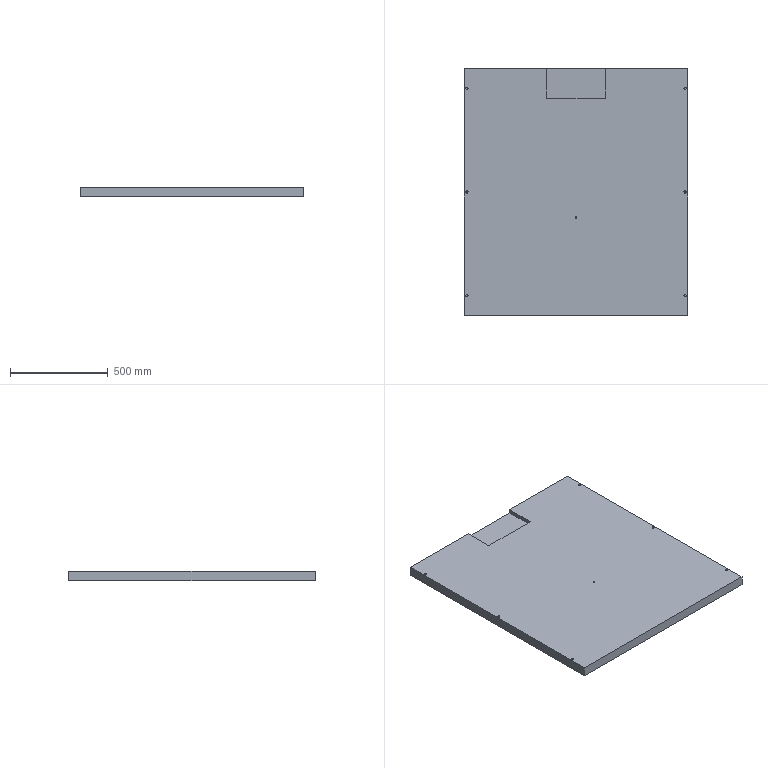Part | SolidWorks | features ICE 2, Extrusion 1 | 1 solid | 31 faces | box 1140 x 1260 x 50 mm | volume 70907025 mm3 | plane 17 | cylinder 14 | commonest cylinder face diameters 11 x12 10 x2
STEP:
#1=CARTESIAN_POINT('',(-563.,-530.,30.));
#2=VERTEX_POINT('',#1);
#3=CARTESIAN_POINT('',(-552.,-530.,30.));
#4=VERTEX_POINT('',#3);
#5=CARTESIAN_POINT('',(-557.5,-530.,30.));
#6=DIRECTION('',(0.,0.,1.));
#7=DIRECTION('',(-1.,0.,0.));
#8=AXIS2_PLACEMENT_3D('',#5,#6,#7);
#9=CIRCLE('',#8,5.5);
#10=EDGE_CURVE('',#2,#4,#9,.T.);
#11=ORIENTED_EDGE('',*,*,#10,.F.);
#12=CARTESIAN_POINT('',(-563.,-530.,50.));
#13=VERTEX_POINT('',#12);
#14=CARTESIAN_POINT('',(-563.,-530.,30.));
#15=DIRECTION('',(0.,0.,1.));
#16=VECTOR('',#15,1000.);
#17=LINE('',#14,#16);
#18=EDGE_CURVE('',#2,#13,#17,.T.);
#19=ORIENTED_EDGE('',*,*,#18,.T.);
#20=CARTESIAN_POINT('',(-552.,-530.,50.));
#21=VERTEX_POINT('',#20);
#22=CARTESIAN_POINT('',(-557.5,-530.,50.));
#23=DIRECTION('',(0.,0.,1.));
#24=DIRECTION('',(-1.,0.,0.));
#25=AXIS2_PLACEMENT_3D('',#22,#23,#24);
#26=CIRCLE('',#25,5.5);
#27=EDGE_CURVE('',#13,#21,#26,.T.);
#28=ORIENTED_EDGE('',*,*,#27,.T.);
#29=CARTESIAN_POINT('',(-552.,-530.,30.));
#30=DIRECTION('',(0.,0.,1.));
#31=VECTOR('',#30,1000.);
#32=LINE('',#29,#31);
#33=EDGE_CURVE('',#4,#21,#32,.T.);
#34=ORIENTED_EDGE('',*,*,#33,.F.);
#35=EDGE_LOOP('',(#11,#19,#28,#34));
#36=FACE_OUTER_BOUND('',#35,.T.);
#37=CARTESIAN_POINT('',(-557.5,-530.,30.));
#38=DIRECTION('',(0.,0.,1.));
#39=DIRECTION('',(1.,0.,0.));
#40=AXIS2_PLACEMENT_3D('',#37,#38,#39);
#41=CYLINDRICAL_SURFACE('',#40,5.5);
#42=ADVANCED_FACE('',(#36),#41,.F.);
#43=CARTESIAN_POINT('',(-563.,0.,30.));
#44=VERTEX_POINT('',#43);
#45=CARTESIAN_POINT('',(-552.,0.,30.));
#46=VERTEX_POINT('',#45);
#47=CARTESIAN_POINT('',(-557.5,0.,30.));
#48=DIRECTION('',(0.,0.,1.));
#49=DIRECTION('',(-1.,0.,0.));
#50=AXIS2_PLACEMENT_3D('',#47,#48,#49);
#51=CIRCLE('',#50,5.5);
#52=EDGE_CURVE('',#44,#46,#51,.T.);
#53=ORIENTED_EDGE('',*,*,#52,.F.);
#54=CARTESIAN_POINT('',(-563.,0.,50.));
#55=VERTEX_POINT('',#54);
#56=CARTESIAN_POINT('',(-563.,0.,30.));
#57=DIRECTION('',(0.,0.,1.));
#58=VECTOR('',#57,1000.);
#59=LINE('',#56,#58);
#60=EDGE_CURVE('',#44,#55,#59,.T.);
#61=ORIENTED_EDGE('',*,*,#60,.T.);
#62=CARTESIAN_POINT('',(-552.,0.,50.));
#63=VERTEX_POINT('',#62);
#64=CARTESIAN_POINT('',(-557.5,0.,50.));
#65=DIRECTION('',(0.,0.,1.));
#66=DIRECTION('',(-1.,0.,0.));
#67=AXIS2_PLACEMENT_3D('',#64,#65,#66);
#68=CIRCLE('',#67,5.5);
#69=EDGE_CURVE('',#55,#63,#68,.T.);
#70=ORIENTED_EDGE('',*,*,#69,.T.);
#71=CARTESIAN_POINT('',(-552.,0.,30.));
#72=DIRECTION('',(0.,0.,1.));
#73=VECTOR('',#72,1000.);
#74=LINE('',#71,#73);
#75=EDGE_CURVE('',#46,#63,#74,.T.);
#76=ORIENTED_EDGE('',*,*,#75,.F.);
#77=EDGE_LOOP('',(#53,#61,#70,#76));
#78=FACE_OUTER_BOUND('',#77,.T.);
#79=CARTESIAN_POINT('',(-557.5,0.,30.));
#80=DIRECTION('',(0.,0.,1.));
#81=DIRECTION('',(1.,0.,0.));
#82=AXIS2_PLACEMENT_3D('',#79,#80,#81);
#83=CYLINDRICAL_SURFACE('',#82,5.5);
#84=ADVANCED_FACE('',(#78),#83,.F.);
#85=CARTESIAN_POINT('',(-563.,530.,30.));
#86=VERTEX_POINT('',#85);
#87=CARTESIAN_POINT('',(-552.,530.,30.));
#88=VERTEX_POINT('',#87);
#89=CARTESIAN_POINT('',(-557.5,530.,30.));
#90=DIRECTION('',(0.,0.,1.));
#91=DIRECTION('',(-1.,0.,0.));
#92=AXIS2_PLACEMENT_3D('',#89,#90,#91);
#93=CIRCLE('',#92,5.5);
#94=EDGE_CURVE('',#86,#88,#93,.T.);
#95=ORIENTED_EDGE('',*,*,#94,.F.);
#96=CARTESIAN_POINT('',(-563.,530.,50.));
#97=VERTEX_POINT('',#96);
#98=CARTESIAN_POINT('',(-563.,530.,30.));
#99=DIRECTION('',(0.,0.,1.));
#100=VECTOR('',#99,1000.);
#101=LINE('',#98,#100);
#102=EDGE_CURVE('',#86,#97,#101,.T.);
#103=ORIENTED_EDGE('',*,*,#102,.T.);
#104=CARTESIAN_POINT('',(-552.,530.,50.));
#105=VERTEX_POINT('',#104);
#106=CARTESIAN_POINT('',(-557.5,530.,50.));
#107=DIRECTION('',(0.,0.,1.));
#108=DIRECTION('',(-1.,0.,0.));
#109=AXIS2_PLACEMENT_3D('',#106,#107,#108);
#110=CIRCLE('',#109,5.5);
#111=EDGE_CURVE('',#97,#105,#110,.T.);
#112=ORIENTED_EDGE('',*,*,#111,.T.);
#113=CARTESIAN_POINT('',(-552.,530.,30.));
#114=DIRECTION('',(0.,0.,1.));
#115=VECTOR('',#114,1000.);
#116=LINE('',#113,#115);
#117=EDGE_CURVE('',#88,#105,#116,.T.);
#118=ORIENTED_EDGE('',*,*,#117,.F.);
#119=EDGE_LOOP('',(#95,#103,#112,#118));
#120=FACE_OUTER_BOUND('',#119,.T.);
#121=CARTESIAN_POINT('',(-557.5,530.,30.));
#122=DIRECTION('',(0.,0.,1.));
#123=DIRECTION('',(1.,0.,0.));
#124=AXIS2_PLACEMENT_3D('',#121,#122,#123);
#125=CYLINDRICAL_SURFACE('',#124,5.5);
#126=ADVANCED_FACE('',(#120),#125,.F.);
#127=CARTESIAN_POINT('',(552.,530.,30.));
#128=VERTEX_POINT('',#127);
#129=CARTESIAN_POINT('',(563.,530.,30.));
#130=VERTEX_POINT('',#129);
#131=CARTESIAN_POINT('',(557.5,530.,30.));
#132=DIRECTION('',(0.,0.,1.));
#133=DIRECTION('',(1.,0.,0.));
#134=AXIS2_PLACEMENT_3D('',#131,#132,#133);
#135=CIRCLE('',#134,5.5);
#136=EDGE_CURVE('',#128,#130,#135,.T.);
#137=ORIENTED_EDGE('',*,*,#136,.F.);
#138=CARTESIAN_POINT('',(552.,530.,50.));
#139=VERTEX_POINT('',#138);
#140=CARTESIAN_POINT('',(552.,530.,30.));
#141=DIRECTION('',(0.,0.,1.));
#142=VECTOR('',#141,1000.);
#143=LINE('',#140,#142);
#144=EDGE_CURVE('',#128,#139,#143,.T.);
#145=ORIENTED_EDGE('',*,*,#144,.T.);
#146=CARTESIAN_POINT('',(563.,530.,50.));
#147=VERTEX_POINT('',#146);
#148=CARTESIAN_POINT('',(557.5,530.,50.));
#149=DIRECTION('',(0.,0.,1.));
#150=DIRECTION('',(1.,0.,0.));
#151=AXIS2_PLACEMENT_3D('',#148,#149,#150);
#152=CIRCLE('',#151,5.5);
#153=EDGE_CURVE('',#139,#147,#152,.T.);
#154=ORIENTED_EDGE('',*,*,#153,.T.);
#155=CARTESIAN_POINT('',(563.,530.,30.));
#156=DIRECTION('',(0.,0.,1.));
#157=VECTOR('',#156,1000.);
#158=LINE('',#155,#157);
#159=EDGE_CURVE('',#130,#147,#158,.T.);
#160=ORIENTED_EDGE('',*,*,#159,.F.);
#161=EDGE_LOOP('',(#137,#145,#154,#160));
#162=FACE_OUTER_BOUND('',#161,.T.);
#163=CARTESIAN_POINT('',(557.5,530.,30.));
#164=DIRECTION('',(0.,0.,1.));
#165=DIRECTION('',(1.,0.,0.));
#166=AXIS2_PLACEMENT_3D('',#163,#164,#165);
#167=CYLINDRICAL_SURFACE('',#166,5.5);
#168=ADVANCED_FACE('',(#162),#167,.F.);
#169=CARTESIAN_POINT('',(552.,0.,30.));
#170=VERTEX_POINT('',#169);
#171=CARTESIAN_POINT('',(563.,0.,30.));
#172=VERTEX_POINT('',#171);
#173=CARTESIAN_POINT('',(557.5,0.,30.));
#174=DIRECTION('',(0.,0.,1.));
#175=DIRECTION('',(1.,0.,0.));
#176=AXIS2_PLACEMENT_3D('',#173,#174,#175);
#177=CIRCLE('',#176,5.5);
#178=EDGE_CURVE('',#170,#172,#177,.T.);
#179=ORIENTED_EDGE('',*,*,#178,.F.);
#180=CARTESIAN_POINT('',(552.,0.,50.));
#181=VERTEX_POINT('',#180);
#182=CARTESIAN_POINT('',(552.,0.,30.));
#183=DIRECTION('',(0.,0.,1.));
#184=VECTOR('',#183,1000.);
#185=LINE('',#182,#184);
#186=EDGE_CURVE('',#170,#181,#185,.T.);
#187=ORIENTED_EDGE('',*,*,#186,.T.);
#188=CARTESIAN_POINT('',(563.,0.,50.));
#189=VERTEX_POINT('',#188);
#190=CARTESIAN_POINT('',(557.5,0.,50.));
#191=DIRECTION('',(0.,0.,1.));
#192=DIRECTION('',(1.,0.,0.));
#193=AXIS2_PLACEMENT_3D('',#190,#191,#192);
#194=CIRCLE('',#193,5.5);
#195=EDGE_CURVE('',#181,#189,#194,.T.);
#196=ORIENTED_EDGE('',*,*,#195,.T.);
#197=CARTESIAN_POINT('',(563.,0.,30.));
#198=DIRECTION('',(0.,0.,1.));
#199=VECTOR('',#198,1000.);
#200=LINE('',#197,#199);
#201=EDGE_CURVE('',#172,#189,#200,.T.);
#202=ORIENTED_EDGE('',*,*,#201,.F.);
#203=EDGE_LOOP('',(#179,#187,#196,#202));
#204=FACE_OUTER_BOUND('',#203,.T.);
#205=CARTESIAN_POINT('',(557.5,0.,30.));
#206=DIRECTION('',(0.,0.,1.));
#207=DIRECTION('',(1.,0.,0.));
#208=AXIS2_PLACEMENT_3D('',#205,#206,#207);
#209=CYLINDRICAL_SURFACE('',#208,5.5);
#210=ADVANCED_FACE('',(#204),#209,.F.);
#211=CARTESIAN_POINT('',(552.,-530.,30.));
#212=VERTEX_POINT('',#211);
#213=CARTESIAN_POINT('',(563.,-530.,30.));
#214=VERTEX_POINT('',#213);
#215=CARTESIAN_POINT('',(557.5,-530.,30.));
#216=DIRECTION('',(0.,0.,1.));
#217=DIRECTION('',(1.,0.,0.));
#218=AXIS2_PLACEMENT_3D('',#215,#216,#217);
#219=CIRCLE('',#218,5.5);
#220=EDGE_CURVE('',#212,#214,#219,.T.);
#221=ORIENTED_EDGE('',*,*,#220,.F.);
#222=CARTESIAN_POINT('',(552.,-530.,50.));
#223=VERTEX_POINT('',#222);
#224=CARTESIAN_POINT('',(552.,-530.,30.));
#225=DIRECTION('',(0.,0.,1.));
#226=VECTOR('',#225,1000.);
#227=LINE('',#224,#226);
#228=EDGE_CURVE('',#212,#223,#227,.T.);
#229=ORIENTED_EDGE('',*,*,#228,.T.);
#230=CARTESIAN_POINT('',(563.,-530.,50.));
#231=VERTEX_POINT('',#230);
#232=CARTESIAN_POINT('',(557.5,-530.,50.));
#233=DIRECTION('',(0.,0.,1.));
#234=DIRECTION('',(1.,0.,0.));
#235=AXIS2_PLACEMENT_3D('',#232,#233,#234);
#236=CIRCLE('',#235,5.5);
#237=EDGE_CURVE('',#223,#231,#236,.T.);
#238=ORIENTED_EDGE('',*,*,#237,.T.);
#239=CARTESIAN_POINT('',(563.,-530.,30.));
#240=DIRECTION('',(0.,0.,1.));
#241=VECTOR('',#240,1000.);
#242=LINE('',#239,#241);
#243=EDGE_CURVE('',#214,#231,#242,.T.);
#244=ORIENTED_EDGE('',*,*,#243,.F.);
#245=EDGE_LOOP('',(#221,#229,#238,#244));
#246=FACE_OUTER_BOUND('',#245,.T.);
#247=CARTESIAN_POINT('',(557.5,-530.,30.));
#248=DIRECTION('',(0.,0.,1.));
#249=DIRECTION('',(1.,0.,0.));
#250=AXIS2_PLACEMENT_3D('',#247,#248,#249);
#251=CYLINDRICAL_SURFACE('',#250,5.5);
#252=ADVANCED_FACE('',(#246),#251,.F.);
#253=CARTESIAN_POINT('',(-5.,-130.,30.));
#254=VERTEX_POINT('',#253);
#255=CARTESIAN_POINT('',(5.,-130.,30.));
#256=VERTEX_POINT('',#255);
#257=CARTESIAN_POINT('',(0.,-130.,30.));
#258=DIRECTION('',(0.,0.,1.));
#259=DIRECTION('',(1.,0.,0.));
#260=AXIS2_PLACEMENT_3D('',#257,#258,#259);
#261=CIRCLE('',#260,5.);
#262=EDGE_CURVE('',#254,#256,#261,.T.);
#263=ORIENTED_EDGE('',*,*,#262,.F.);
#264=CARTESIAN_POINT('',(-5.,-130.,50.));
#265=VERTEX_POINT('',#264);
#266=CARTESIAN_POINT('',(-5.,-130.,30.));
#267=DIRECTION('',(0.,0.,1.));
#268=VECTOR('',#267,1000.);
#269=LINE('',#266,#268);
#270=EDGE_CURVE('',#254,#265,#269,.T.);
#271=ORIENTED_EDGE('',*,*,#270,.T.);
#272=CARTESIAN_POINT('',(5.,-130.,50.));
#273=VERTEX_POINT('',#272);
#274=CARTESIAN_POINT('',(0.,-130.,50.));
#275=DIRECTION('',(0.,0.,1.));
#276=DIRECTION('',(1.,0.,0.));
#277=AXIS2_PLACEMENT_3D('',#274,#275,#276);
#278=CIRCLE('',#277,5.);
#279=EDGE_CURVE('',#265,#273,#278,.T.);
#280=ORIENTED_EDGE('',*,*,#279,.T.);
#281=CARTESIAN_POINT('',(5.,-130.,30.));
#282=DIRECTION('',(0.,0.,1.));
#283=VECTOR('',#282,1000.);
#284=LINE('',#281,#283);
#285=EDGE_CURVE('',#256,#273,#284,.T.);
#286=ORIENTED_EDGE('',*,*,#285,.F.);
#287=EDGE_LOOP('',(#263,#271,#280,#286));
#288=FACE_OUTER_BOUND('',#287,.T.);
#289=CARTESIAN_POINT('',(0.,-130.,30.));
#290=DIRECTION('',(0.,0.,1.));
#291=DIRECTION('',(1.,0.,0.));
#292=AXIS2_PLACEMENT_3D('',#289,#290,#291);
#293=CYLINDRICAL_SURFACE('',#292,5.);
#294=ADVANCED_FACE('',(#288),#293,.F.);
#295=CARTESIAN_POINT('',(570.,-630.,0.));
#296=VERTEX_POINT('',#295);
#297=CARTESIAN_POINT('',(570.,630.,0.));
#298=VERTEX_POINT('',#297);
#299=CARTESIAN_POINT('',(570.,630.,0.));
#300=DIRECTION('',(0.,1.,0.));
#301=VECTOR('',#300,1000.);
#302=LINE('',#299,#301);
#303=EDGE_CURVE('',#296,#298,#302,.T.);
#304=ORIENTED_EDGE('',*,*,#303,.T.);
#305=CARTESIAN_POINT('',(570.,630.,50.));
#306=VERTEX_POINT('',#305);
#307=CARTESIAN_POINT('',(570.,630.,50.));
#308=DIRECTION('',(0.,0.,-1.));
#309=VECTOR('',#308,1000.);
#310=LINE('',#307,#309);
#311=EDGE_CURVE('',#306,#298,#310,.T.);
#312=ORIENTED_EDGE('',*,*,#311,.F.);
#313=CARTESIAN_POINT('',(570.,-630.,50.));
#314=VERTEX_POINT('',#313);
#315=CARTESIAN_POINT('',(570.,630.,50.));
#316=DIRECTION('',(0.,1.,0.));
#317=VECTOR('',#316,1000.);
#318=LINE('',#315,#317);
#319=EDGE_CURVE('',#314,#306,#318,.T.);
#320=ORIENTED_EDGE('',*,*,#319,.F.);
#321=CARTESIAN_POINT('',(570.,-630.,50.));
#322=DIRECTION('',(0.,0.,-1.));
#323=VECTOR('',#322,1000.);
#324=LINE('',#321,#323);
#325=EDGE_CURVE('',#314,#296,#324,.T.);
#326=ORIENTED_EDGE('',*,*,#325,.T.);
#327=EDGE_LOOP('',(#304,#312,#320,#326));
#328=FACE_OUTER_BOUND('',#327,.T.);
#329=CARTESIAN_POINT('',(570.,630.,50.));
#330=DIRECTION('',(-1.,0.,0.));
#331=DIRECTION('',(0.,-1.,0.));
#332=AXIS2_PLACEMENT_3D('',#329,#330,#331);
#333=PLANE('',#332);
#334=ADVANCED_FACE('',(#328),#333,.F.);
#335=CARTESIAN_POINT('',(150.,630.,30.));
#336=VERTEX_POINT('',#335);
#337=CARTESIAN_POINT('',(-150.,630.,30.));
#338=VERTEX_POINT('',#337);
#339=CARTESIAN_POINT('',(-570.,630.,30.));
#340=DIRECTION('',(-1.,0.,0.));
#341=VECTOR('',#340,1000.);
#342=LINE('',#339,#341);
#343=EDGE_CURVE('',#336,#338,#342,.T.);
#344=ORIENTED_EDGE('',*,*,#343,.F.);
#345=CARTESIAN_POINT('',(150.,630.,50.));
#346=VERTEX_POINT('',#345);
#347=CARTESIAN_POINT('',(150.,630.,50.));
#348=DIRECTION('',(0.,0.,1.));
#349=VECTOR('',#348,1000.);
#350=LINE('',#347,#349);
#351=EDGE_CURVE('',#336,#346,#350,.T.);
#352=ORIENTED_EDGE('',*,*,#351,.T.);
#353=CARTESIAN_POINT('',(-570.,630.,50.));
#354=DIRECTION('',(-1.,0.,0.));
#355=VECTOR('',#354,1000.);
#356=LINE('',#353,#355);
#357=EDGE_CURVE('',#306,#346,#356,.T.);
#358=ORIENTED_EDGE('',*,*,#357,.F.);
#359=ORIENTED_EDGE('',*,*,#311,.T.);
#360=CARTESIAN_POINT('',(-570.,630.,0.));
#361=VERTEX_POINT('',#360);
#362=CARTESIAN_POINT('',(-570.,630.,0.));
#363=DIRECTION('',(-1.,0.,0.));
#364=VECTOR('',#363,1000.);
#365=LINE('',#362,#364);
#366=EDGE_CURVE('',#298,#361,#365,.T.);
#367=ORIENTED_EDGE('',*,*,#366,.T.);
#368=CARTESIAN_POINT('',(-570.,630.,50.));
#369=VERTEX_POINT('',#368);
#370=CARTESIAN_POINT('',(-570.,630.,50.));
#371=DIRECTION('',(0.,0.,-1.));
#372=VECTOR('',#371,1000.);
#373=LINE('',#370,#372);
#374=EDGE_CURVE('',#369,#361,#373,.T.);
#375=ORIENTED_EDGE('',*,*,#374,.F.);
#376=CARTESIAN_POINT('',(-150.,630.,50.));
#377=VERTEX_POINT('',#376);
#378=CARTESIAN_POINT('',(-570.,630.,50.));
#379=DIRECTION('',(-1.,0.,0.));
#380=VECTOR('',#379,1000.);
#381=LINE('',#378,#380);
#382=EDGE_CURVE('',#377,#369,#381,.T.);
#383=ORIENTED_EDGE('',*,*,#382,.F.);
#384=CARTESIAN_POINT('',(-150.,630.,50.));
#385=DIRECTION('',(0.,0.,-1.));
#386=VECTOR('',#385,1000.);
#387=LINE('',#384,#386);
#388=EDGE_CURVE('',#377,#338,#387,.T.);
#389=ORIENTED_EDGE('',*,*,#388,.T.);
#390=EDGE_LOOP('',(#344,#352,#358,#359,#367,#375,#383,#389));
#391=FACE_OUTER_BOUND('',#390,.T.);
#392=CARTESIAN_POINT('',(-570.,630.,50.));
#393=DIRECTION('',(0.,-1.,0.));
#394=DIRECTION('',(0.,0.,-1.));
#395=AXIS2_PLACEMENT_3D('',#392,#393,#394);
#396=PLANE('',#395);
#397=ADVANCED_FACE('',(#391),#396,.F.);
#398=CARTESIAN_POINT('',(-570.,-630.,0.));
#399=VERTEX_POINT('',#398);
#400=CARTESIAN_POINT('',(-570.,630.,0.));
#401=DIRECTION('',(0.,-1.,0.));
#402=VECTOR('',#401,1000.);
#403=LINE('',#400,#402);
#404=EDGE_CURVE('',#361,#399,#403,.T.);
#405=ORIENTED_EDGE('',*,*,#404,.T.);
#406=CARTESIAN_POINT('',(-570.,-630.,50.));
#407=VERTEX_POINT('',#406);
#408=CARTESIAN_POINT('',(-570.,-630.,50.));
#409=DIRECTION('',(0.,0.,-1.));
#410=VECTOR('',#409,1000.);
#411=LINE('',#408,#410);
#412=EDGE_CURVE('',#407,#399,#411,.T.);
#413=ORIENTED_EDGE('',*,*,#412,.F.);
#414=CARTESIAN_POINT('',(-570.,630.,50.));
#415=DIRECTION('',(0.,-1.,0.));
#416=VECTOR('',#415,1000.);
#417=LINE('',#414,#416);
#418=EDGE_CURVE('',#369,#407,#417,.T.);
#419=ORIENTED_EDGE('',*,*,#418,.F.);
#420=ORIENTED_EDGE('',*,*,#374,.T.);
#421=EDGE_LOOP('',(#405,#413,#419,#420));
#422=FACE_OUTER_BOUND('',#421,.T.);
#423=CARTESIAN_POINT('',(-570.,630.,50.));
#424=DIRECTION('',(1.,0.,0.));
#425=DIRECTION('',(0.,1.,0.));
#426=AXIS2_PLACEMENT_3D('',#423,#424,#425);
#427=PLANE('',#426);
#428=ADVANCED_FACE('',(#422),#427,.F.);
#429=CARTESIAN_POINT('',(-570.,-630.,0.));
#430=DIRECTION('',(1.,0.,0.));
#431=VECTOR('',#430,1000.);
#432=LINE('',#429,#431);
#433=EDGE_CURVE('',#399,#296,#432,.T.);
#434=ORIENTED_EDGE('',*,*,#433,.T.);
#435=ORIENTED_EDGE('',*,*,#325,.F.);
#436=CARTESIAN_POINT('',(-570.,-630.,50.));
#437=DIRECTION('',(1.,0.,0.));
#438=VECTOR('',#437,1000.);
#439=LINE('',#436,#438);
#440=EDGE_CURVE('',#407,#314,#439,.T.);
#441=ORIENTED_EDGE('',*,*,#440,.F.);
#442=ORIENTED_EDGE('',*,*,#412,.T.);
#443=EDGE_LOOP('',(#434,#435,#441,#442));
#444=FACE_OUTER_BOUND('',#443,.T.);
#445=CARTESIAN_POINT('',(-570.,-630.,50.));
#446=DIRECTION('',(0.,1.,0.));
#447=DIRECTION('',(0.,0.,1.));
#448=AXIS2_PLACEMENT_3D('',#445,#446,#447);
#449=PLANE('',#448);
#450=ADVANCED_FACE('',(#444),#449,.F.);
#451=CARTESIAN_POINT('',(-557.5,-530.,50.));
#452=DIRECTION('',(0.,0.,1.));
#453=DIRECTION('',(-1.,0.,0.));
#454=AXIS2_PLACEMENT_3D('',#451,#452,#453);
#455=CIRCLE('',#454,5.5);
#456=EDGE_CURVE('',#21,#13,#455,.T.);
#457=ORIENTED_EDGE('',*,*,#456,.F.);
#458=ORIENTED_EDGE('',*,*,#27,.F.);
#459=EDGE_LOOP('',(#457,#458));
#460=FACE_BOUND('',#459,.T.);
#461=CARTESIAN_POINT('',(-557.5,0.,50.));
#462=DIRECTION('',(0.,0.,1.));
#463=DIRECTION('',(-1.,0.,0.));
#464=AXIS2_PLACEMENT_3D('',#461,#462,#463);
#465=CIRCLE('',#464,5.5);
#466=EDGE_CURVE('',#63,#55,#465,.T.);
#467=ORIENTED_EDGE('',*,*,#466,.F.);
#468=ORIENTED_EDGE('',*,*,#69,.F.);
#469=EDGE_LOOP('',(#467,#468));
#470=FACE_BOUND('',#469,.T.);
#471=CARTESIAN_POINT('',(-557.5,530.,50.));
#472=DIRECTION('',(0.,0.,1.));
#473=DIRECTION('',(-1.,0.,0.));
#474=AXIS2_PLACEMENT_3D('',#471,#472,#473);
#475=CIRCLE('',#474,5.5);
#476=EDGE_CURVE('',#105,#97,#475,.T.);
#477=ORIENTED_EDGE('',*,*,#476,.F.);
#478=ORIENTED_EDGE('',*,*,#111,.F.);
#479=EDGE_LOOP('',(#477,#478));
#480=FACE_BOUND('',#479,.T.);
#481=CARTESIAN_POINT('',(557.5,530.,50.));
#482=DIRECTION('',(0.,0.,1.));
#483=DIRECTION('',(1.,0.,0.));
#484=AXIS2_PLACEMENT_3D('',#481,#482,#483);
#485=CIRCLE('',#484,5.5);
#486=EDGE_CURVE('',#147,#139,#485,.T.);
#487=ORIENTED_EDGE('',*,*,#486,.F.);
#488=ORIENTED_EDGE('',*,*,#153,.F.);
#489=EDGE_LOOP('',(#487,#488));
#490=FACE_BOUND('',#489,.T.);
#491=CARTESIAN_POINT('',(557.5,0.,50.));
#492=DIRECTION('',(0.,0.,1.));
#493=DIRECTION('',(1.,0.,0.));
#494=AXIS2_PLACEMENT_3D('',#491,#492,#493);
#495=CIRCLE('',#494,5.5);
#496=EDGE_CURVE('',#189,#181,#495,.T.);
#497=ORIENTED_EDGE('',*,*,#496,.F.);
#498=ORIENTED_EDGE('',*,*,#195,.F.);
#499=EDGE_LOOP('',(#497,#498));
#500=FACE_BOUND('',#499,.T.);
#501=CARTESIAN_POINT('',(557.5,-530.,50.));
#502=DIRECTION('',(0.,0.,1.));
#503=DIRECTION('',(1.,0.,0.));
#504=AXIS2_PLACEMENT_3D('',#501,#502,#503);
#505=CIRCLE('',#504,5.5);
#506=EDGE_CURVE('',#231,#223,#505,.T.);
#507=ORIENTED_EDGE('',*,*,#506,.F.);
#508=ORIENTED_EDGE('',*,*,#237,.F.);
#509=EDGE_LOOP('',(#507,#508));
#510=FACE_BOUND('',#509,.T.);
#511=CARTESIAN_POINT('',(0.,-130.,50.));
#512=DIRECTION('',(0.,0.,1.));
#513=DIRECTION('',(1.,0.,0.));
#514=AXIS2_PLACEMENT_3D('',#511,#512,#513);
#515=CIRCLE('',#514,5.);
#516=EDGE_CURVE('',#273,#265,#515,.T.);
#517=ORIENTED_EDGE('',*,*,#516,.F.);
#518=ORIENTED_EDGE('',*,*,#279,.F.);
#519=EDGE_LOOP('',(#517,#518));
#520=FACE_BOUND('',#519,.T.);
#521=CARTESIAN_POINT('',(150.,480.,50.));
#522=VERTEX_POINT('',#521);
#523=CARTESIAN_POINT('',(150.,780.,50.));
#524=DIRECTION('',(0.,1.,0.));
#525=VECTOR('',#524,1000.);
#526=LINE('',#523,#525);
#527=EDGE_CURVE('',#522,#346,#526,.T.);
#528=ORIENTED_EDGE('',*,*,#527,.F.);
#529=CARTESIAN_POINT('',(-150.,480.,50.));
#530=VERTEX_POINT('',#529);
#531=CARTESIAN_POINT('',(-150.,480.,50.));
#532=DIRECTION('',(1.,0.,0.));
#533=VECTOR('',#532,1000.);
#534=LINE('',#531,#533);
#535=EDGE_CURVE('',#530,#522,#534,.T.);
#536=ORIENTED_EDGE('',*,*,#535,.F.);
#537=CARTESIAN_POINT('',(-150.,0.,50.));
#538=DIRECTION('',(0.,-1.,0.));
#539=VECTOR('',#538,1000.);
#540=LINE('',#537,#539);
#541=EDGE_CURVE('',#377,#530,#540,.T.);
#542=ORIENTED_EDGE('',*,*,#541,.F.);
#543=ORIENTED_EDGE('',*,*,#382,.T.);
#544=ORIENTED_EDGE('',*,*,#418,.T.);
#545=ORIENTED_EDGE('',*,*,#440,.T.);
#546=ORIENTED_EDGE('',*,*,#319,.T.);
#547=ORIENTED_EDGE('',*,*,#357,.T.);
#548=EDGE_LOOP('',(#528,#536,#542,#543,#544,#545,#546,#547));
#549=FACE_OUTER_BOUND('',#548,.T.);
#550=CARTESIAN_POINT('',(0.,0.,50.));
#551=DIRECTION('',(0.,0.,1.));
#552=DIRECTION('',(1.,0.,0.));
#553=AXIS2_PLACEMENT_3D('',#550,#551,#552);
#554=PLANE('',#553);
#555=ADVANCED_FACE('',(#460,#470,#480,#490,#500,#510,#520,#549),#554,.T.);
#556=ORIENTED_EDGE('',*,*,#303,.F.);
#557=ORIENTED_EDGE('',*,*,#433,.F.);
#558=ORIENTED_EDGE('',*,*,#404,.F.);
#559=ORIENTED_EDGE('',*,*,#366,.F.);
#560=EDGE_LOOP('',(#556,#557,#558,#559));
#561=FACE_OUTER_BOUND('',#560,.T.);
#562=CARTESIAN_POINT('',(0.,0.,0.));
#563=DIRECTION('',(0.,0.,1.));
#564=DIRECTION('',(1.,0.,0.));
#565=AXIS2_PLACEMENT_3D('',#562,#563,#564);
#566=PLANE('',#565);
#567=ADVANCED_FACE('',(#561),#566,.F.);
#568=ORIENTED_EDGE('',*,*,#343,.T.);
#569=CARTESIAN_POINT('',(-150.,480.,30.));
#570=VERTEX_POINT('',#569);
#571=CARTESIAN_POINT('',(-150.,780.,30.));
#572=DIRECTION('',(0.,-1.,0.));
#573=VECTOR('',#572,1000.);
#574=LINE('',#571,#573);
#575=EDGE_CURVE('',#338,#570,#574,.T.);
#576=ORIENTED_EDGE('',*,*,#575,.T.);
#577=CARTESIAN_POINT('',(150.,480.,30.));
#578=VERTEX_POINT('',#577);
#579=CARTESIAN_POINT('',(-150.,480.,30.));
#580=DIRECTION('',(1.,0.,0.));
#581=VECTOR('',#580,1000.);
#582=LINE('',#579,#581);
#583=EDGE_CURVE('',#570,#578,#582,.T.);
#584=ORIENTED_EDGE('',*,*,#583,.T.);
#585=CARTESIAN_POINT('',(150.,780.,30.));
#586=DIRECTION('',(0.,1.,0.));
#587=VECTOR('',#586,1000.);
#588=LINE('',#585,#587);
#589=EDGE_CURVE('',#578,#336,#588,.T.);
#590=ORIENTED_EDGE('',*,*,#589,.T.);
#591=EDGE_LOOP('',(#568,#576,#584,#590));
#592=FACE_OUTER_BOUND('',#591,.T.);
#593=CARTESIAN_POINT('',(0.,0.,30.));
#594=DIRECTION('',(0.,0.,1.));
#595=DIRECTION('',(1.,0.,0.));
#596=AXIS2_PLACEMENT_3D('',#593,#594,#595);
#597=PLANE('',#596);
#598=ADVANCED_FACE('',(#592),#597,.T.);
#599=ORIENTED_EDGE('',*,*,#589,.F.);
#600=CARTESIAN_POINT('',(150.,480.,30.));
#601=DIRECTION('',(0.,0.,1.));
#602=VECTOR('',#601,1000.);
#603=LINE('',#600,#602);
#604=EDGE_CURVE('',#578,#522,#603,.T.);
#605=ORIENTED_EDGE('',*,*,#604,.T.);
#606=ORIENTED_EDGE('',*,*,#527,.T.);
#607=ORIENTED_EDGE('',*,*,#351,.F.);
#608=EDGE_LOOP('',(#599,#605,#606,#607));
#609=FACE_OUTER_BOUND('',#608,.T.);
#610=CARTESIAN_POINT('',(150.,780.,30.));
#611=DIRECTION('',(1.,0.,0.));
#612=DIRECTION('',(0.,1.,0.));
#613=AXIS2_PLACEMENT_3D('',#610,#611,#612);
#614=PLANE('',#613);
#615=ADVANCED_FACE('',(#609),#614,.F.);
#616=ORIENTED_EDGE('',*,*,#541,.T.);
#617=CARTESIAN_POINT('',(-150.,480.,30.));
#618=DIRECTION('',(0.,0.,1.));
#619=VECTOR('',#618,1000.);
#620=LINE('',#617,#619);
#621=EDGE_CURVE('',#570,#530,#620,.T.);
#622=ORIENTED_EDGE('',*,*,#621,.F.);
#623=ORIENTED_EDGE('',*,*,#575,.F.);
#624=ORIENTED_EDGE('',*,*,#388,.F.);
#625=EDGE_LOOP('',(#616,#622,#623,#624));
#626=FACE_OUTER_BOUND('',#625,.T.);
#627=CARTESIAN_POINT('',(-150.,780.,30.));
#628=DIRECTION('',(-1.,0.,0.));
#629=DIRECTION('',(0.,-1.,0.));
#630=AXIS2_PLACEMENT_3D('',#627,#628,#629);
#631=PLANE('',#630);
#632=ADVANCED_FACE('',(#626),#631,.F.);
#633=ORIENTED_EDGE('',*,*,#535,.T.);
#634=ORIENTED_EDGE('',*,*,#604,.F.);
#635=ORIENTED_EDGE('',*,*,#583,.F.);
#636=ORIENTED_EDGE('',*,*,#621,.T.);
#637=EDGE_LOOP('',(#633,#634,#635,#636));
#638=FACE_OUTER_BOUND('',#637,.T.);
#639=CARTESIAN_POINT('',(-150.,480.,30.));
#640=DIRECTION('',(0.,-1.,0.));
#641=DIRECTION('',(0.,0.,-1.));
#642=AXIS2_PLACEMENT_3D('',#639,#640,#641);
#643=PLANE('',#642);
#644=ADVANCED_FACE('',(#638),#643,.F.);
#645=ORIENTED_EDGE('',*,*,#270,.F.);
#646=CARTESIAN_POINT('',(0.,-130.,30.));
#647=DIRECTION('',(0.,0.,1.));
#648=DIRECTION('',(1.,0.,0.));
#649=AXIS2_PLACEMENT_3D('',#646,#647,#648);
#650=CIRCLE('',#649,5.);
#651=EDGE_CURVE('',#256,#254,#650,.T.);
#652=ORIENTED_EDGE('',*,*,#651,.F.);
#653=ORIENTED_EDGE('',*,*,#285,.T.);
#654=ORIENTED_EDGE('',*,*,#516,.T.);
#655=EDGE_LOOP('',(#645,#652,#653,#654));
#656=FACE_OUTER_BOUND('',#655,.T.);
#657=CARTESIAN_POINT('',(0.,-130.,30.));
#658=DIRECTION('',(0.,0.,1.));
#659=DIRECTION('',(1.,0.,0.));
#660=AXIS2_PLACEMENT_3D('',#657,#658,#659);
#661=CYLINDRICAL_SURFACE('',#660,5.);
#662=ADVANCED_FACE('',(#656),#661,.F.);
#663=ORIENTED_EDGE('',*,*,#651,.T.);
#664=ORIENTED_EDGE('',*,*,#262,.T.);
#665=EDGE_LOOP('',(#663,#664));
#666=FACE_OUTER_BOUND('',#665,.T.);
#667=CARTESIAN_POINT('',(0.,-130.,30.));
#668=DIRECTION('',(0.,0.,1.));
#669=DIRECTION('',(1.,0.,0.));
#670=AXIS2_PLACEMENT_3D('',#667,#668,#669);
#671=PLANE('',#670);
#672=ADVANCED_FACE('',(#666),#671,.T.);
#673=ORIENTED_EDGE('',*,*,#228,.F.);
#674=CARTESIAN_POINT('',(557.5,-530.,30.));
#675=DIRECTION('',(0.,0.,1.));
#676=DIRECTION('',(1.,0.,0.));
#677=AXIS2_PLACEMENT_3D('',#674,#675,#676);
#678=CIRCLE('',#677,5.5);
#679=EDGE_CURVE('',#214,#212,#678,.T.);
#680=ORIENTED_EDGE('',*,*,#679,.F.);
#681=ORIENTED_EDGE('',*,*,#243,.T.);
#682=ORIENTED_EDGE('',*,*,#506,.T.);
#683=EDGE_LOOP('',(#673,#680,#681,#682));
#684=FACE_OUTER_BOUND('',#683,.T.);
#685=CARTESIAN_POINT('',(557.5,-530.,30.));
#686=DIRECTION('',(0.,0.,1.));
#687=DIRECTION('',(1.,0.,0.));
#688=AXIS2_PLACEMENT_3D('',#685,#686,#687);
#689=CYLINDRICAL_SURFACE('',#688,5.5);
#690=ADVANCED_FACE('',(#684),#689,.F.);
#691=ORIENTED_EDGE('',*,*,#679,.T.);
#692=ORIENTED_EDGE('',*,*,#220,.T.);
#693=EDGE_LOOP('',(#691,#692));
#694=FACE_OUTER_BOUND('',#693,.T.);
#695=CARTESIAN_POINT('',(557.5,-530.,30.));
#696=DIRECTION('',(0.,0.,1.));
#697=DIRECTION('',(1.,0.,0.));
#698=AXIS2_PLACEMENT_3D('',#695,#696,#697);
#699=PLANE('',#698);
#700=ADVANCED_FACE('',(#694),#699,.T.);
#701=ORIENTED_EDGE('',*,*,#186,.F.);
#702=CARTESIAN_POINT('',(557.5,0.,30.));
#703=DIRECTION('',(0.,0.,1.));
#704=DIRECTION('',(1.,0.,0.));
#705=AXIS2_PLACEMENT_3D('',#702,#703,#704);
#706=CIRCLE('',#705,5.5);
#707=EDGE_CURVE('',#172,#170,#706,.T.);
#708=ORIENTED_EDGE('',*,*,#707,.F.);
#709=ORIENTED_EDGE('',*,*,#201,.T.);
#710=ORIENTED_EDGE('',*,*,#496,.T.);
#711=EDGE_LOOP('',(#701,#708,#709,#710));
#712=FACE_OUTER_BOUND('',#711,.T.);
#713=CARTESIAN_POINT('',(557.5,0.,30.));
#714=DIRECTION('',(0.,0.,1.));
#715=DIRECTION('',(1.,0.,0.));
#716=AXIS2_PLACEMENT_3D('',#713,#714,#715);
#717=CYLINDRICAL_SURFACE('',#716,5.5);
#718=ADVANCED_FACE('',(#712),#717,.F.);
#719=ORIENTED_EDGE('',*,*,#707,.T.);
#720=ORIENTED_EDGE('',*,*,#178,.T.);
#721=EDGE_LOOP('',(#719,#720));
#722=FACE_OUTER_BOUND('',#721,.T.);
#723=CARTESIAN_POINT('',(557.5,0.,30.));
#724=DIRECTION('',(0.,0.,1.));
#725=DIRECTION('',(1.,0.,0.));
#726=AXIS2_PLACEMENT_3D('',#723,#724,#725);
#727=PLANE('',#726);
#728=ADVANCED_FACE('',(#722),#727,.T.);
#729=ORIENTED_EDGE('',*,*,#144,.F.);
#730=CARTESIAN_POINT('',(557.5,530.,30.));
#731=DIRECTION('',(0.,0.,1.));
#732=DIRECTION('',(1.,0.,0.));
#733=AXIS2_PLACEMENT_3D('',#730,#731,#732);
#734=CIRCLE('',#733,5.5);
#735=EDGE_CURVE('',#130,#128,#734,.T.);
#736=ORIENTED_EDGE('',*,*,#735,.F.);
#737=ORIENTED_EDGE('',*,*,#159,.T.);
#738=ORIENTED_EDGE('',*,*,#486,.T.);
#739=EDGE_LOOP('',(#729,#736,#737,#738));
#740=FACE_OUTER_BOUND('',#739,.T.);
#741=CARTESIAN_POINT('',(557.5,530.,30.));
#742=DIRECTION('',(0.,0.,1.));
#743=DIRECTION('',(1.,0.,0.));
#744=AXIS2_PLACEMENT_3D('',#741,#742,#743);
#745=CYLINDRICAL_SURFACE('',#744,5.5);
#746=ADVANCED_FACE('',(#740),#745,.F.);
#747=ORIENTED_EDGE('',*,*,#735,.T.);
#748=ORIENTED_EDGE('',*,*,#136,.T.);
#749=EDGE_LOOP('',(#747,#748));
#750=FACE_OUTER_BOUND('',#749,.T.);
#751=CARTESIAN_POINT('',(557.5,530.,30.));
#752=DIRECTION('',(0.,0.,1.));
#753=DIRECTION('',(1.,0.,0.));
#754=AXIS2_PLACEMENT_3D('',#751,#752,#753);
#755=PLANE('',#754);
#756=ADVANCED_FACE('',(#750),#755,.T.);
#757=ORIENTED_EDGE('',*,*,#102,.F.);
#758=CARTESIAN_POINT('',(-557.5,530.,30.));
#759=DIRECTION('',(0.,0.,1.));
#760=DIRECTION('',(-1.,0.,0.));
#761=AXIS2_PLACEMENT_3D('',#758,#759,#760);
#762=CIRCLE('',#761,5.5);
#763=EDGE_CURVE('',#88,#86,#762,.T.);
#764=ORIENTED_EDGE('',*,*,#763,.F.);
#765=ORIENTED_EDGE('',*,*,#117,.T.);
#766=ORIENTED_EDGE('',*,*,#476,.T.);
#767=EDGE_LOOP('',(#757,#764,#765,#766));
#768=FACE_OUTER_BOUND('',#767,.T.);
#769=CARTESIAN_POINT('',(-557.5,530.,30.));
#770=DIRECTION('',(0.,0.,1.));
#771=DIRECTION('',(1.,0.,0.));
#772=AXIS2_PLACEMENT_3D('',#769,#770,#771);
#773=CYLINDRICAL_SURFACE('',#772,5.5);
#774=ADVANCED_FACE('',(#768),#773,.F.);
#775=ORIENTED_EDGE('',*,*,#763,.T.);
#776=ORIENTED_EDGE('',*,*,#94,.T.);
#777=EDGE_LOOP('',(#775,#776));
#778=FACE_OUTER_BOUND('',#777,.T.);
#779=CARTESIAN_POINT('',(-557.5,530.,30.));
#780=DIRECTION('',(0.,0.,-1.));
#781=DIRECTION('',(-1.,0.,0.));
#782=AXIS2_PLACEMENT_3D('',#779,#780,#781);
#783=PLANE('',#782);
#784=ADVANCED_FACE('',(#778),#783,.F.);
#785=ORIENTED_EDGE('',*,*,#60,.F.);
#786=CARTESIAN_POINT('',(-557.5,0.,30.));
#787=DIRECTION('',(0.,0.,1.));
#788=DIRECTION('',(-1.,0.,0.));
#789=AXIS2_PLACEMENT_3D('',#786,#787,#788);
#790=CIRCLE('',#789,5.5);
#791=EDGE_CURVE('',#46,#44,#790,.T.);
#792=ORIENTED_EDGE('',*,*,#791,.F.);
#793=ORIENTED_EDGE('',*,*,#75,.T.);
#794=ORIENTED_EDGE('',*,*,#466,.T.);
#795=EDGE_LOOP('',(#785,#792,#793,#794));
#796=FACE_OUTER_BOUND('',#795,.T.);
#797=CARTESIAN_POINT('',(-557.5,0.,30.));
#798=DIRECTION('',(0.,0.,1.));
#799=DIRECTION('',(1.,0.,0.));
#800=AXIS2_PLACEMENT_3D('',#797,#798,#799);
#801=CYLINDRICAL_SURFACE('',#800,5.5);
#802=ADVANCED_FACE('',(#796),#801,.F.);
#803=ORIENTED_EDGE('',*,*,#791,.T.);
#804=ORIENTED_EDGE('',*,*,#52,.T.);
#805=EDGE_LOOP('',(#803,#804));
#806=FACE_OUTER_BOUND('',#805,.T.);
#807=CARTESIAN_POINT('',(-557.5,0.,30.));
#808=DIRECTION('',(0.,0.,-1.));
#809=DIRECTION('',(-1.,0.,0.));
#810=AXIS2_PLACEMENT_3D('',#807,#808,#809);
#811=PLANE('',#810);
#812=ADVANCED_FACE('',(#806),#811,.F.);
#813=ORIENTED_EDGE('',*,*,#18,.F.);
#814=CARTESIAN_POINT('',(-557.5,-530.,30.));
#815=DIRECTION('',(0.,0.,1.));
#816=DIRECTION('',(-1.,0.,0.));
#817=AXIS2_PLACEMENT_3D('',#814,#815,#816);
#818=CIRCLE('',#817,5.5);
#819=EDGE_CURVE('',#4,#2,#818,.T.);
#820=ORIENTED_EDGE('',*,*,#819,.F.);
#821=ORIENTED_EDGE('',*,*,#33,.T.);
#822=ORIENTED_EDGE('',*,*,#456,.T.);
#823=EDGE_LOOP('',(#813,#820,#821,#822));
#824=FACE_OUTER_BOUND('',#823,.T.);
#825=CARTESIAN_POINT('',(-557.5,-530.,30.));
#826=DIRECTION('',(0.,0.,1.));
#827=DIRECTION('',(1.,0.,0.));
#828=AXIS2_PLACEMENT_3D('',#825,#826,#827);
#829=CYLINDRICAL_SURFACE('',#828,5.5);
#830=ADVANCED_FACE('',(#824),#829,.F.);
#831=ORIENTED_EDGE('',*,*,#819,.T.);
#832=ORIENTED_EDGE('',*,*,#10,.T.);
#833=EDGE_LOOP('',(#831,#832));
#834=FACE_OUTER_BOUND('',#833,.T.);
#835=CARTESIAN_POINT('',(-557.5,-530.,30.));
#836=DIRECTION('',(0.,0.,-1.));
#837=DIRECTION('',(-1.,0.,0.));
#838=AXIS2_PLACEMENT_3D('',#835,#836,#837);
#839=PLANE('',#838);
#840=ADVANCED_FACE('',(#834),#839,.F.);
#841=CLOSED_SHELL('',(#42,#84,#126,#168,#210,#252,#294,#334,#397,#428,#450,#555,#567,#598,#615,#632,#644,#662,#672,#690,#700,#718,#728,#746,#756,#774,#784,#802,#812,#830,#840));
#842=MANIFOLD_SOLID_BREP('',#841);
#843=CARTESIAN_POINT('',(0.,0.,0.));
#844=DIRECTION('',(0.,0.,1.));
#845=DIRECTION('',(1.,0.,0.));
#846=AXIS2_PLACEMENT_3D('',#843,#844,#845);
#847=(LENGTH_UNIT()NAMED_UNIT(*)SI_UNIT(.MILLI.,.METRE.));
#848=UNCERTAINTY_MEASURE_WITH_UNIT(LENGTH_MEASURE(0.00001),#847,'','');
#849=(NAMED_UNIT(*)PLANE_ANGLE_UNIT()SI_UNIT($,.RADIAN.));
#850=(NAMED_UNIT(*)SI_UNIT($,.STERADIAN.)SOLID_ANGLE_UNIT());
#851=(GEOMETRIC_REPRESENTATION_CONTEXT(3)GLOBAL_UNCERTAINTY_ASSIGNED_CONTEXT((#848))GLOBAL_UNIT_ASSIGNED_CONTEXT((#847,#849,#850))REPRESENTATION_CONTEXT('',''));
#852=ADVANCED_BREP_SHAPE_REPRESENTATION('',(#842,#846),#851);